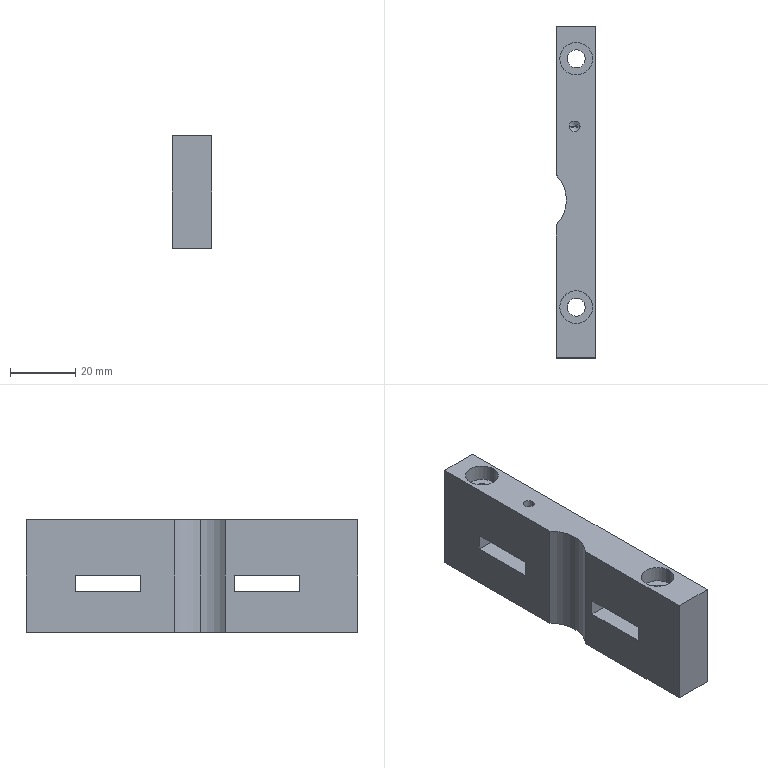Part | STEP file | side block 4 | 1 solid | 48 faces | box 12.1 x 101.5 x 34.5 mm | volume 36196 mm3 | cylinder 20 | plane 18 | cone 10 | commonest cylinder face diameters 3.3 x10 5.5 x4 10 x4 22 x2